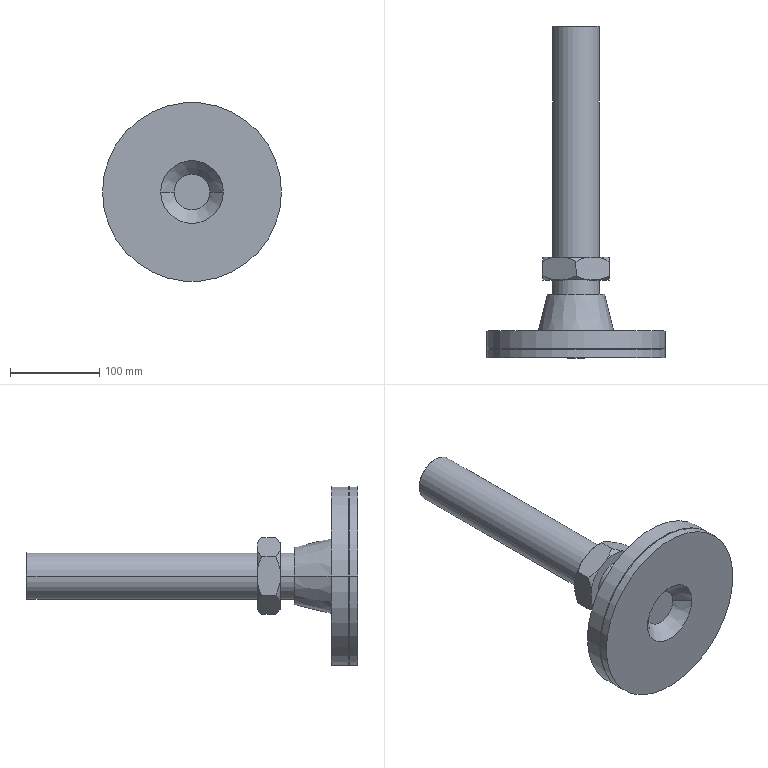Part | SolidWorks | features ICE 2, RevCut 2, Chamfer 1, Revolution 1 | 1 solid | 43 faces | box 200 x 371 x 200 mm | volume 1786955 mm3 | cone 22 | plane 13 | cylinder 8 | commonest cylinder face diameters 52 x4 200 x4
STEP:
#1=CARTESIAN_POINT('',(-25.,371.,0.));
#2=VERTEX_POINT('',#1);
#3=CARTESIAN_POINT('',(25.,371.,0.));
#4=VERTEX_POINT('',#3);
#5=CARTESIAN_POINT('',(0.,371.,0.));
#6=DIRECTION('',(0.,1.,0.));
#7=DIRECTION('',(1.,0.,0.));
#8=AXIS2_PLACEMENT_3D('',#5,#6,#7);
#9=CIRCLE('',#8,25.);
#10=EDGE_CURVE('',#2,#4,#9,.T.);
#11=ORIENTED_EDGE('',*,*,#10,.F.);
#12=CARTESIAN_POINT('',(-26.,370.,0.));
#13=VERTEX_POINT('',#12);
#14=CARTESIAN_POINT('',(-25.,371.,0.));
#15=DIRECTION('',(-0.7071,-0.7071,0.));
#16=VECTOR('',#15,1000.);
#17=LINE('',#14,#16);
#18=EDGE_CURVE('',#2,#13,#17,.T.);
#19=ORIENTED_EDGE('',*,*,#18,.T.);
#20=CARTESIAN_POINT('',(26.,370.,0.));
#21=VERTEX_POINT('',#20);
#22=CARTESIAN_POINT('',(0.,370.,0.));
#23=DIRECTION('',(0.,-1.,0.));
#24=DIRECTION('',(1.,0.,0.));
#25=AXIS2_PLACEMENT_3D('',#22,#23,#24);
#26=CIRCLE('',#25,26.);
#27=EDGE_CURVE('',#21,#13,#26,.T.);
#28=ORIENTED_EDGE('',*,*,#27,.F.);
#29=CARTESIAN_POINT('',(25.,371.,0.));
#30=DIRECTION('',(0.7071,-0.7071,0.));
#31=VECTOR('',#30,1000.);
#32=LINE('',#29,#31);
#33=EDGE_CURVE('',#4,#21,#32,.T.);
#34=ORIENTED_EDGE('',*,*,#33,.F.);
#35=EDGE_LOOP('',(#11,#19,#28,#34));
#36=FACE_OUTER_BOUND('',#35,.T.);
#37=CARTESIAN_POINT('',(0.,371.,0.));
#38=DIRECTION('',(0.,-1.,0.));
#39=DIRECTION('',(1.,0.,0.));
#40=AXIS2_PLACEMENT_3D('',#37,#38,#39);
#41=CONICAL_SURFACE('',#40,25.,0.7854);
#42=ADVANCED_FACE('',(#36),#41,.T.);
#43=CARTESIAN_POINT('',(-26.,112.6,0.));
#44=VERTEX_POINT('',#43);
#45=CARTESIAN_POINT('',(26.,112.6,0.));
#46=VERTEX_POINT('',#45);
#47=CARTESIAN_POINT('',(0.,112.6,0.));
#48=DIRECTION('',(0.,1.,0.));
#49=DIRECTION('',(-1.,0.,0.));
#50=AXIS2_PLACEMENT_3D('',#47,#48,#49);
#51=CIRCLE('',#50,26.);
#52=EDGE_CURVE('',#44,#46,#51,.T.);
#53=ORIENTED_EDGE('',*,*,#52,.T.);
#54=CARTESIAN_POINT('',(26.,371.,0.));
#55=DIRECTION('',(0.,1.,0.));
#56=VECTOR('',#55,1000.);
#57=LINE('',#54,#56);
#58=EDGE_CURVE('',#46,#21,#57,.T.);
#59=ORIENTED_EDGE('',*,*,#58,.T.);
#60=ORIENTED_EDGE('',*,*,#27,.T.);
#61=CARTESIAN_POINT('',(-26.,371.,0.));
#62=DIRECTION('',(0.,1.,0.));
#63=VECTOR('',#62,1000.);
#64=LINE('',#61,#63);
#65=EDGE_CURVE('',#44,#13,#64,.T.);
#66=ORIENTED_EDGE('',*,*,#65,.F.);
#67=EDGE_LOOP('',(#53,#59,#60,#66));
#68=FACE_OUTER_BOUND('',#67,.T.);
#69=CARTESIAN_POINT('',(0.,371.,0.));
#70=DIRECTION('',(0.,1.,0.));
#71=DIRECTION('',(-1.,0.,0.));
#72=AXIS2_PLACEMENT_3D('',#69,#70,#71);
#73=CYLINDRICAL_SURFACE('',#72,26.);
#74=ADVANCED_FACE('',(#68),#73,.T.);
#75=CARTESIAN_POINT('',(20.,15.,0.));
#76=VERTEX_POINT('',#75);
#77=CARTESIAN_POINT('',(-20.,15.,0.));
#78=VERTEX_POINT('',#77);
#79=CARTESIAN_POINT('',(0.,15.,0.));
#80=DIRECTION('',(0.,1.,0.));
#81=DIRECTION('',(-1.,0.,0.));
#82=AXIS2_PLACEMENT_3D('',#79,#80,#81);
#83=CIRCLE('',#82,20.);
#84=EDGE_CURVE('',#76,#78,#83,.T.);
#85=ORIENTED_EDGE('',*,*,#84,.T.);
#86=CARTESIAN_POINT('',(-35.,0.,0.));
#87=VERTEX_POINT('',#86);
#88=CARTESIAN_POINT('',(-20.,15.,0.));
#89=DIRECTION('',(-0.7071,-0.7071,0.));
#90=VECTOR('',#89,1000.);
#91=LINE('',#88,#90);
#92=EDGE_CURVE('',#78,#87,#91,.T.);
#93=ORIENTED_EDGE('',*,*,#92,.T.);
#94=CARTESIAN_POINT('',(35.,0.,0.));
#95=VERTEX_POINT('',#94);
#96=CARTESIAN_POINT('',(0.,0.,0.));
#97=DIRECTION('',(0.,1.,0.));
#98=DIRECTION('',(-1.,0.,0.));
#99=AXIS2_PLACEMENT_3D('',#96,#97,#98);
#100=CIRCLE('',#99,35.);
#101=EDGE_CURVE('',#95,#87,#100,.T.);
#102=ORIENTED_EDGE('',*,*,#101,.F.);
#103=CARTESIAN_POINT('',(20.,15.,0.));
#104=DIRECTION('',(0.7071,-0.7071,0.));
#105=VECTOR('',#104,1000.);
#106=LINE('',#103,#105);
#107=EDGE_CURVE('',#76,#95,#106,.T.);
#108=ORIENTED_EDGE('',*,*,#107,.F.);
#109=EDGE_LOOP('',(#85,#93,#102,#108));
#110=FACE_OUTER_BOUND('',#109,.T.);
#111=CARTESIAN_POINT('',(0.,15.,0.));
#112=DIRECTION('',(0.,-1.,0.));
#113=DIRECTION('',(1.,0.,0.));
#114=AXIS2_PLACEMENT_3D('',#111,#112,#113);
#115=CONICAL_SURFACE('',#114,20.,0.7854);
#116=ADVANCED_FACE('',(#110),#115,.F.);
#117=CARTESIAN_POINT('',(-32.,71.,0.));
#118=VERTEX_POINT('',#117);
#119=CARTESIAN_POINT('',(32.,71.,0.));
#120=VERTEX_POINT('',#119);
#121=CARTESIAN_POINT('',(0.,71.,0.));
#122=DIRECTION('',(0.,1.,0.));
#123=DIRECTION('',(-1.,0.,0.));
#124=AXIS2_PLACEMENT_3D('',#121,#122,#123);
#125=CIRCLE('',#124,32.);
#126=EDGE_CURVE('',#118,#120,#125,.T.);
#127=ORIENTED_EDGE('',*,*,#126,.F.);
#128=CARTESIAN_POINT('',(-42.,30.,0.));
#129=VERTEX_POINT('',#128);
#130=CARTESIAN_POINT('',(-42.,30.,0.));
#131=DIRECTION('',(-0.237,-0.9715,0.));
#132=VECTOR('',#131,1000.);
#133=LINE('',#130,#132);
#134=EDGE_CURVE('',#118,#129,#133,.T.);
#135=ORIENTED_EDGE('',*,*,#134,.T.);
#136=CARTESIAN_POINT('',(42.,30.,0.));
#137=VERTEX_POINT('',#136);
#138=CARTESIAN_POINT('',(0.,30.,0.));
#139=DIRECTION('',(0.,1.,0.));
#140=DIRECTION('',(-1.,0.,0.));
#141=AXIS2_PLACEMENT_3D('',#138,#139,#140);
#142=CIRCLE('',#141,42.);
#143=EDGE_CURVE('',#129,#137,#142,.T.);
#144=ORIENTED_EDGE('',*,*,#143,.T.);
#145=CARTESIAN_POINT('',(42.,30.,0.));
#146=DIRECTION('',(0.237,-0.9715,0.));
#147=VECTOR('',#146,1000.);
#148=LINE('',#145,#147);
#149=EDGE_CURVE('',#120,#137,#148,.T.);
#150=ORIENTED_EDGE('',*,*,#149,.F.);
#151=EDGE_LOOP('',(#127,#135,#144,#150));
#152=FACE_OUTER_BOUND('',#151,.T.);
#153=CARTESIAN_POINT('',(0.,30.,0.));
#154=DIRECTION('',(0.,-1.,0.));
#155=DIRECTION('',(1.,0.,0.));
#156=AXIS2_PLACEMENT_3D('',#153,#154,#155);
#157=CONICAL_SURFACE('',#156,42.,0.2392);
#158=ADVANCED_FACE('',(#152),#157,.T.);
#159=CARTESIAN_POINT('',(-100.,10.5,0.));
#160=VERTEX_POINT('',#159);
#161=CARTESIAN_POINT('',(100.,10.5,0.));
#162=VERTEX_POINT('',#161);
#163=CARTESIAN_POINT('',(0.,10.5,0.));
#164=DIRECTION('',(0.,1.,0.));
#165=DIRECTION('',(-1.,0.,0.));
#166=AXIS2_PLACEMENT_3D('',#163,#164,#165);
#167=CIRCLE('',#166,100.);
#168=EDGE_CURVE('',#160,#162,#167,.T.);
#169=ORIENTED_EDGE('',*,*,#168,.T.);
#170=CARTESIAN_POINT('',(100.,30.,0.));
#171=VERTEX_POINT('',#170);
#172=CARTESIAN_POINT('',(100.,371.,0.));
#173=DIRECTION('',(0.,1.,0.));
#174=VECTOR('',#173,1000.);
#175=LINE('',#172,#174);
#176=EDGE_CURVE('',#162,#171,#175,.T.);
#177=ORIENTED_EDGE('',*,*,#176,.T.);
#178=CARTESIAN_POINT('',(-100.,30.,0.));
#179=VERTEX_POINT('',#178);
#180=CARTESIAN_POINT('',(0.,30.,0.));
#181=DIRECTION('',(0.,1.,0.));
#182=DIRECTION('',(-1.,0.,0.));
#183=AXIS2_PLACEMENT_3D('',#180,#181,#182);
#184=CIRCLE('',#183,100.);
#185=EDGE_CURVE('',#179,#171,#184,.T.);
#186=ORIENTED_EDGE('',*,*,#185,.F.);
#187=CARTESIAN_POINT('',(-100.,371.,0.));
#188=DIRECTION('',(0.,1.,0.));
#189=VECTOR('',#188,1000.);
#190=LINE('',#187,#189);
#191=EDGE_CURVE('',#160,#179,#190,.T.);
#192=ORIENTED_EDGE('',*,*,#191,.F.);
#193=EDGE_LOOP('',(#169,#177,#186,#192));
#194=FACE_OUTER_BOUND('',#193,.T.);
#195=CARTESIAN_POINT('',(0.,371.,0.));
#196=DIRECTION('',(0.,1.,0.));
#197=DIRECTION('',(-1.,0.,0.));
#198=AXIS2_PLACEMENT_3D('',#195,#196,#197);
#199=CYLINDRICAL_SURFACE('',#198,100.);
#200=ADVANCED_FACE('',(#194),#199,.T.);
#201=CARTESIAN_POINT('',(-99.5,10.,0.));
#202=VERTEX_POINT('',#201);
#203=CARTESIAN_POINT('',(99.5,10.,0.));
#204=VERTEX_POINT('',#203);
#205=CARTESIAN_POINT('',(0.,10.,0.));
#206=DIRECTION('',(0.,1.,0.));
#207=DIRECTION('',(-1.,0.,0.));
#208=AXIS2_PLACEMENT_3D('',#205,#206,#207);
#209=CIRCLE('',#208,99.5);
#210=EDGE_CURVE('',#202,#204,#209,.T.);
#211=ORIENTED_EDGE('',*,*,#210,.T.);
#212=CARTESIAN_POINT('',(99.5,10.,0.));
#213=DIRECTION('',(0.7071,0.7071,0.));
#214=VECTOR('',#213,1000.);
#215=LINE('',#212,#214);
#216=EDGE_CURVE('',#204,#162,#215,.T.);
#217=ORIENTED_EDGE('',*,*,#216,.T.);
#218=ORIENTED_EDGE('',*,*,#168,.F.);
#219=CARTESIAN_POINT('',(-99.5,10.,0.));
#220=DIRECTION('',(-0.7071,0.7071,0.));
#221=VECTOR('',#220,1000.);
#222=LINE('',#219,#221);
#223=EDGE_CURVE('',#202,#160,#222,.T.);
#224=ORIENTED_EDGE('',*,*,#223,.F.);
#225=EDGE_LOOP('',(#211,#217,#218,#224));
#226=FACE_OUTER_BOUND('',#225,.T.);
#227=CARTESIAN_POINT('',(0.,10.,0.));
#228=DIRECTION('',(0.,1.,0.));
#229=DIRECTION('',(-1.,0.,0.));
#230=AXIS2_PLACEMENT_3D('',#227,#228,#229);
#231=CONICAL_SURFACE('',#230,99.5,0.7854);
#232=ADVANCED_FACE('',(#226),#231,.T.);
#233=ORIENTED_EDGE('',*,*,#210,.F.);
#234=CARTESIAN_POINT('',(-100.,9.5,0.));
#235=VERTEX_POINT('',#234);
#236=CARTESIAN_POINT('',(-100.,9.5,0.));
#237=DIRECTION('',(-0.7071,-0.7071,0.));
#238=VECTOR('',#237,1000.);
#239=LINE('',#236,#238);
#240=EDGE_CURVE('',#202,#235,#239,.T.);
#241=ORIENTED_EDGE('',*,*,#240,.T.);
#242=CARTESIAN_POINT('',(100.,9.5,0.));
#243=VERTEX_POINT('',#242);
#244=CARTESIAN_POINT('',(0.,9.5,0.));
#245=DIRECTION('',(0.,1.,0.));
#246=DIRECTION('',(-1.,0.,0.));
#247=AXIS2_PLACEMENT_3D('',#244,#245,#246);
#248=CIRCLE('',#247,100.);
#249=EDGE_CURVE('',#235,#243,#248,.T.);
#250=ORIENTED_EDGE('',*,*,#249,.T.);
#251=CARTESIAN_POINT('',(100.,9.5,0.));
#252=DIRECTION('',(0.7071,-0.7071,0.));
#253=VECTOR('',#252,1000.);
#254=LINE('',#251,#253);
#255=EDGE_CURVE('',#204,#243,#254,.T.);
#256=ORIENTED_EDGE('',*,*,#255,.F.);
#257=EDGE_LOOP('',(#233,#241,#250,#256));
#258=FACE_OUTER_BOUND('',#257,.T.);
#259=CARTESIAN_POINT('',(0.,9.5,0.));
#260=DIRECTION('',(0.,-1.,0.));
#261=DIRECTION('',(1.,0.,0.));
#262=AXIS2_PLACEMENT_3D('',#259,#260,#261);
#263=CONICAL_SURFACE('',#262,100.,0.7854);
#264=ADVANCED_FACE('',(#258),#263,.T.);
#265=CARTESIAN_POINT('',(-100.,0.,0.));
#266=VERTEX_POINT('',#265);
#267=CARTESIAN_POINT('',(100.,0.,0.));
#268=VERTEX_POINT('',#267);
#269=CARTESIAN_POINT('',(0.,0.,0.));
#270=DIRECTION('',(0.,1.,0.));
#271=DIRECTION('',(-1.,0.,0.));
#272=AXIS2_PLACEMENT_3D('',#269,#270,#271);
#273=CIRCLE('',#272,100.);
#274=EDGE_CURVE('',#266,#268,#273,.T.);
#275=ORIENTED_EDGE('',*,*,#274,.T.);
#276=CARTESIAN_POINT('',(100.,371.,0.));
#277=DIRECTION('',(0.,1.,0.));
#278=VECTOR('',#277,1000.);
#279=LINE('',#276,#278);
#280=EDGE_CURVE('',#268,#243,#279,.T.);
#281=ORIENTED_EDGE('',*,*,#280,.T.);
#282=ORIENTED_EDGE('',*,*,#249,.F.);
#283=CARTESIAN_POINT('',(-100.,371.,0.));
#284=DIRECTION('',(0.,1.,0.));
#285=VECTOR('',#284,1000.);
#286=LINE('',#283,#285);
#287=EDGE_CURVE('',#266,#235,#286,.T.);
#288=ORIENTED_EDGE('',*,*,#287,.F.);
#289=EDGE_LOOP('',(#275,#281,#282,#288));
#290=FACE_OUTER_BOUND('',#289,.T.);
#291=CARTESIAN_POINT('',(0.,371.,0.));
#292=DIRECTION('',(0.,1.,0.));
#293=DIRECTION('',(-1.,0.,0.));
#294=AXIS2_PLACEMENT_3D('',#291,#292,#293);
#295=CYLINDRICAL_SURFACE('',#294,100.);
#296=ADVANCED_FACE('',(#290),#295,.T.);
#297=CARTESIAN_POINT('',(-26.,71.,0.));
#298=VERTEX_POINT('',#297);
#299=CARTESIAN_POINT('',(26.,71.,0.));
#300=VERTEX_POINT('',#299);
#301=CARTESIAN_POINT('',(0.,71.,0.));
#302=DIRECTION('',(0.,1.,0.));
#303=DIRECTION('',(-1.,0.,0.));
#304=AXIS2_PLACEMENT_3D('',#301,#302,#303);
#305=CIRCLE('',#304,26.);
#306=EDGE_CURVE('',#298,#300,#305,.T.);
#307=ORIENTED_EDGE('',*,*,#306,.T.);
#308=CARTESIAN_POINT('',(26.,87.,0.));
#309=VERTEX_POINT('',#308);
#310=CARTESIAN_POINT('',(26.,371.,0.));
#311=DIRECTION('',(0.,1.,0.));
#312=VECTOR('',#311,1000.);
#313=LINE('',#310,#312);
#314=EDGE_CURVE('',#300,#309,#313,.T.);
#315=ORIENTED_EDGE('',*,*,#314,.T.);
#316=CARTESIAN_POINT('',(-26.,87.,0.));
#317=VERTEX_POINT('',#316);
#318=CARTESIAN_POINT('',(0.,87.,0.));
#319=DIRECTION('',(0.,1.,0.));
#320=DIRECTION('',(0.,0.,1.));
#321=AXIS2_PLACEMENT_3D('',#318,#319,#320);
#322=CIRCLE('',#321,26.);
#323=EDGE_CURVE('',#317,#309,#322,.T.);
#324=ORIENTED_EDGE('',*,*,#323,.F.);
#325=CARTESIAN_POINT('',(-26.,371.,0.));
#326=DIRECTION('',(0.,1.,0.));
#327=VECTOR('',#326,1000.);
#328=LINE('',#325,#327);
#329=EDGE_CURVE('',#298,#317,#328,.T.);
#330=ORIENTED_EDGE('',*,*,#329,.F.);
#331=EDGE_LOOP('',(#307,#315,#324,#330));
#332=FACE_OUTER_BOUND('',#331,.T.);
#333=CARTESIAN_POINT('',(0.,371.,0.));
#334=DIRECTION('',(0.,1.,0.));
#335=DIRECTION('',(-1.,0.,0.));
#336=AXIS2_PLACEMENT_3D('',#333,#334,#335);
#337=CYLINDRICAL_SURFACE('',#336,26.);
#338=ADVANCED_FACE('',(#332),#337,.T.);
#339=ORIENTED_EDGE('',*,*,#52,.F.);
#340=CARTESIAN_POINT('',(0.,112.6,0.));
#341=DIRECTION('',(0.,1.,0.));
#342=DIRECTION('',(-1.,0.,0.));
#343=AXIS2_PLACEMENT_3D('',#340,#341,#342);
#344=CIRCLE('',#343,26.);
#345=EDGE_CURVE('',#46,#44,#344,.T.);
#346=ORIENTED_EDGE('',*,*,#345,.F.);
#347=EDGE_LOOP('',(#339,#346));
#348=FACE_BOUND('',#347,.T.);
#349=CARTESIAN_POINT('',(-24.996,112.6,28.408));
#350=VERTEX_POINT('',#349);
#351=CARTESIAN_POINT('',(-37.1,112.6,7.444));
#352=VERTEX_POINT('',#351);
#353=CARTESIAN_POINT('',(0.,112.6,0.));
#354=DIRECTION('',(0.,-1.,0.));
#355=DIRECTION('',(1.,0.,0.));
#356=AXIS2_PLACEMENT_3D('',#353,#354,#355);
#357=CIRCLE('',#356,37.839);
#358=EDGE_CURVE('',#350,#352,#357,.T.);
#359=ORIENTED_EDGE('',*,*,#358,.F.);
#360=CARTESIAN_POINT('',(-12.104,112.6,35.851));
#361=VERTEX_POINT('',#360);
#362=CARTESIAN_POINT('',(-37.1,112.6,21.42));
#363=DIRECTION('',(0.866,0.,0.5));
#364=VECTOR('',#363,1000.);
#365=LINE('',#362,#364);
#366=EDGE_CURVE('',#350,#361,#365,.T.);
#367=ORIENTED_EDGE('',*,*,#366,.T.);
#368=CARTESIAN_POINT('',(12.104,112.6,35.851));
#369=VERTEX_POINT('',#368);
#370=CARTESIAN_POINT('',(0.,112.6,0.));
#371=DIRECTION('',(0.,-1.,0.));
#372=DIRECTION('',(1.,0.,0.));
#373=AXIS2_PLACEMENT_3D('',#370,#371,#372);
#374=CIRCLE('',#373,37.839);
#375=EDGE_CURVE('',#369,#361,#374,.T.);
#376=ORIENTED_EDGE('',*,*,#375,.F.);
#377=CARTESIAN_POINT('',(24.996,112.6,28.408));
#378=VERTEX_POINT('',#377);
#379=CARTESIAN_POINT('',(0.,112.6,42.839));
#380=DIRECTION('',(0.866,0.,-0.5));
#381=VECTOR('',#380,1000.);
#382=LINE('',#379,#381);
#383=EDGE_CURVE('',#369,#378,#382,.T.);
#384=ORIENTED_EDGE('',*,*,#383,.T.);
#385=CARTESIAN_POINT('',(37.1,112.6,7.444));
#386=VERTEX_POINT('',#385);
#387=CARTESIAN_POINT('',(0.,112.6,0.));
#388=DIRECTION('',(0.,-1.,0.));
#389=DIRECTION('',(1.,0.,0.));
#390=AXIS2_PLACEMENT_3D('',#387,#388,#389);
#391=CIRCLE('',#390,37.839);
#392=EDGE_CURVE('',#386,#378,#391,.T.);
#393=ORIENTED_EDGE('',*,*,#392,.F.);
#394=CARTESIAN_POINT('',(37.1,112.6,-7.444));
#395=VERTEX_POINT('',#394);
#396=CARTESIAN_POINT('',(37.1,112.6,21.42));
#397=DIRECTION('',(0.,0.,-1.));
#398=VECTOR('',#397,1000.);
#399=LINE('',#396,#398);
#400=EDGE_CURVE('',#386,#395,#399,.T.);
#401=ORIENTED_EDGE('',*,*,#400,.T.);
#402=CARTESIAN_POINT('',(24.996,112.6,-28.408));
#403=VERTEX_POINT('',#402);
#404=CARTESIAN_POINT('',(0.,112.6,0.));
#405=DIRECTION('',(0.,-1.,0.));
#406=DIRECTION('',(1.,0.,0.));
#407=AXIS2_PLACEMENT_3D('',#404,#405,#406);
#408=CIRCLE('',#407,37.839);
#409=EDGE_CURVE('',#403,#395,#408,.T.);
#410=ORIENTED_EDGE('',*,*,#409,.F.);
#411=CARTESIAN_POINT('',(12.104,112.6,-35.851));
#412=VERTEX_POINT('',#411);
#413=CARTESIAN_POINT('',(37.1,112.6,-21.42));
#414=DIRECTION('',(-0.866,0.,-0.5));
#415=VECTOR('',#414,1000.);
#416=LINE('',#413,#415);
#417=EDGE_CURVE('',#403,#412,#416,.T.);
#418=ORIENTED_EDGE('',*,*,#417,.T.);
#419=CARTESIAN_POINT('',(-12.104,112.6,-35.851));
#420=VERTEX_POINT('',#419);
#421=CARTESIAN_POINT('',(0.,112.6,0.));
#422=DIRECTION('',(0.,-1.,0.));
#423=DIRECTION('',(1.,0.,0.));
#424=AXIS2_PLACEMENT_3D('',#421,#422,#423);
#425=CIRCLE('',#424,37.839);
#426=EDGE_CURVE('',#420,#412,#425,.T.);
#427=ORIENTED_EDGE('',*,*,#426,.F.);
#428=CARTESIAN_POINT('',(-24.996,112.6,-28.408));
#429=VERTEX_POINT('',#428);
#430=CARTESIAN_POINT('',(0.,112.6,-42.839));
#431=DIRECTION('',(-0.866,0.,0.5));
#432=VECTOR('',#431,1000.);
#433=LINE('',#430,#432);
#434=EDGE_CURVE('',#420,#429,#433,.T.);
#435=ORIENTED_EDGE('',*,*,#434,.T.);
#436=CARTESIAN_POINT('',(-37.1,112.6,-7.444));
#437=VERTEX_POINT('',#436);
#438=CARTESIAN_POINT('',(0.,112.6,0.));
#439=DIRECTION('',(0.,-1.,0.));
#440=DIRECTION('',(1.,0.,0.));
#441=AXIS2_PLACEMENT_3D('',#438,#439,#440);
#442=CIRCLE('',#441,37.839);
#443=EDGE_CURVE('',#437,#429,#442,.T.);
#444=ORIENTED_EDGE('',*,*,#443,.F.);
#445=CARTESIAN_POINT('',(-37.1,112.6,-21.42));
#446=DIRECTION('',(0.,0.,1.));
#447=VECTOR('',#446,1000.);
#448=LINE('',#445,#447);
#449=EDGE_CURVE('',#437,#352,#448,.T.);
#450=ORIENTED_EDGE('',*,*,#449,.T.);
#451=EDGE_LOOP('',(#359,#367,#376,#384,#393,#401,#410,#418,#427,#435,#444,#450));
#452=FACE_OUTER_BOUND('',#451,.T.);
#453=CARTESIAN_POINT('',(0.,112.6,0.));
#454=DIRECTION('',(0.,1.,0.));
#455=DIRECTION('',(0.,0.,1.));
#456=AXIS2_PLACEMENT_3D('',#453,#454,#455);
#457=PLANE('',#456);
#458=ADVANCED_FACE('',(#348,#452),#457,.T.);
#459=ORIENTED_EDGE('',*,*,#314,.F.);
#460=CARTESIAN_POINT('',(0.,71.,0.));
#461=DIRECTION('',(0.,1.,0.));
#462=DIRECTION('',(-1.,0.,0.));
#463=AXIS2_PLACEMENT_3D('',#460,#461,#462);
#464=CIRCLE('',#463,26.);
#465=EDGE_CURVE('',#300,#298,#464,.T.);
#466=ORIENTED_EDGE('',*,*,#465,.T.);
#467=ORIENTED_EDGE('',*,*,#329,.T.);
#468=CARTESIAN_POINT('',(0.,87.,0.));
#469=DIRECTION('',(0.,1.,0.));
#470=DIRECTION('',(0.,0.,1.));
#471=AXIS2_PLACEMENT_3D('',#468,#469,#470);
#472=CIRCLE('',#471,26.);
#473=EDGE_CURVE('',#309,#317,#472,.T.);
#474=ORIENTED_EDGE('',*,*,#473,.F.);
#475=EDGE_LOOP('',(#459,#466,#467,#474));
#476=FACE_OUTER_BOUND('',#475,.T.);
#477=CARTESIAN_POINT('',(0.,371.,0.));
#478=DIRECTION('',(0.,1.,0.));
#479=DIRECTION('',(-1.,0.,0.));
#480=AXIS2_PLACEMENT_3D('',#477,#478,#479);
#481=CYLINDRICAL_SURFACE('',#480,26.);
#482=ADVANCED_FACE('',(#476),#481,.T.);
#483=ORIENTED_EDGE('',*,*,#280,.F.);
#484=CARTESIAN_POINT('',(0.,0.,0.));
#485=DIRECTION('',(0.,1.,0.));
#486=DIRECTION('',(-1.,0.,0.));
#487=AXIS2_PLACEMENT_3D('',#484,#485,#486);
#488=CIRCLE('',#487,100.);
#489=EDGE_CURVE('',#268,#266,#488,.T.);
#490=ORIENTED_EDGE('',*,*,#489,.T.);
#491=ORIENTED_EDGE('',*,*,#287,.T.);
#492=CARTESIAN_POINT('',(0.,9.5,0.));
#493=DIRECTION('',(0.,1.,0.));
#494=DIRECTION('',(-1.,0.,0.));
#495=AXIS2_PLACEMENT_3D('',#492,#493,#494);
#496=CIRCLE('',#495,100.);
#497=EDGE_CURVE('',#243,#235,#496,.T.);
#498=ORIENTED_EDGE('',*,*,#497,.F.);
#499=EDGE_LOOP('',(#483,#490,#491,#498));
#500=FACE_OUTER_BOUND('',#499,.T.);
#501=CARTESIAN_POINT('',(0.,371.,0.));
#502=DIRECTION('',(0.,1.,0.));
#503=DIRECTION('',(-1.,0.,0.));
#504=AXIS2_PLACEMENT_3D('',#501,#502,#503);
#505=CYLINDRICAL_SURFACE('',#504,100.);
#506=ADVANCED_FACE('',(#500),#505,.T.);
#507=ORIENTED_EDGE('',*,*,#240,.F.);
#508=CARTESIAN_POINT('',(0.,10.,0.));
#509=DIRECTION('',(0.,1.,0.));
#510=DIRECTION('',(-1.,0.,0.));
#511=AXIS2_PLACEMENT_3D('',#508,#509,#510);
#512=CIRCLE('',#511,99.5);
#513=EDGE_CURVE('',#204,#202,#512,.T.);
#514=ORIENTED_EDGE('',*,*,#513,.F.);
#515=ORIENTED_EDGE('',*,*,#255,.T.);
#516=ORIENTED_EDGE('',*,*,#497,.T.);
#517=EDGE_LOOP('',(#507,#514,#515,#516));
#518=FACE_OUTER_BOUND('',#517,.T.);
#519=CARTESIAN_POINT('',(0.,9.5,0.));
#520=DIRECTION('',(0.,-1.,0.));
#521=DIRECTION('',(1.,0.,0.));
#522=AXIS2_PLACEMENT_3D('',#519,#520,#521);
#523=CONICAL_SURFACE('',#522,100.,0.7854);
#524=ADVANCED_FACE('',(#518),#523,.T.);
#525=ORIENTED_EDGE('',*,*,#216,.F.);
#526=ORIENTED_EDGE('',*,*,#513,.T.);
#527=ORIENTED_EDGE('',*,*,#223,.T.);
#528=CARTESIAN_POINT('',(0.,10.5,0.));
#529=DIRECTION('',(0.,1.,0.));
#530=DIRECTION('',(-1.,0.,0.));
#531=AXIS2_PLACEMENT_3D('',#528,#529,#530);
#532=CIRCLE('',#531,100.);
#533=EDGE_CURVE('',#162,#160,#532,.T.);
#534=ORIENTED_EDGE('',*,*,#533,.F.);
#535=EDGE_LOOP('',(#525,#526,#527,#534));
#536=FACE_OUTER_BOUND('',#535,.T.);
#537=CARTESIAN_POINT('',(0.,10.,0.));
#538=DIRECTION('',(0.,1.,0.));
#539=DIRECTION('',(-1.,0.,0.));
#540=AXIS2_PLACEMENT_3D('',#537,#538,#539);
#541=CONICAL_SURFACE('',#540,99.5,0.7854);
#542=ADVANCED_FACE('',(#536),#541,.T.);
#543=ORIENTED_EDGE('',*,*,#176,.F.);
#544=ORIENTED_EDGE('',*,*,#533,.T.);
#545=ORIENTED_EDGE('',*,*,#191,.T.);
#546=CARTESIAN_POINT('',(0.,30.,0.));
#547=DIRECTION('',(0.,1.,0.));
#548=DIRECTION('',(-1.,0.,0.));
#549=AXIS2_PLACEMENT_3D('',#546,#547,#548);
#550=CIRCLE('',#549,100.);
#551=EDGE_CURVE('',#171,#179,#550,.T.);
#552=ORIENTED_EDGE('',*,*,#551,.F.);
#553=EDGE_LOOP('',(#543,#544,#545,#552));
#554=FACE_OUTER_BOUND('',#553,.T.);
#555=CARTESIAN_POINT('',(0.,371.,0.));
#556=DIRECTION('',(0.,1.,0.));
#557=DIRECTION('',(-1.,0.,0.));
#558=AXIS2_PLACEMENT_3D('',#555,#556,#557);
#559=CYLINDRICAL_SURFACE('',#558,100.);
#560=ADVANCED_FACE('',(#554),#559,.T.);
#561=CARTESIAN_POINT('',(0.,30.,0.));
#562=DIRECTION('',(0.,1.,0.));
#563=DIRECTION('',(-1.,0.,0.));
#564=AXIS2_PLACEMENT_3D('',#561,#562,#563);
#565=CIRCLE('',#564,42.);
#566=EDGE_CURVE('',#137,#129,#565,.T.);
#567=ORIENTED_EDGE('',*,*,#566,.F.);
#568=ORIENTED_EDGE('',*,*,#143,.F.);
#569=EDGE_LOOP('',(#567,#568));
#570=FACE_BOUND('',#569,.T.);
#571=ORIENTED_EDGE('',*,*,#185,.T.);
#572=ORIENTED_EDGE('',*,*,#551,.T.);
#573=EDGE_LOOP('',(#571,#572));
#574=FACE_OUTER_BOUND('',#573,.T.);
#575=CARTESIAN_POINT('',(100.,30.,0.));
#576=DIRECTION('',(0.,-1.,0.));
#577=DIRECTION('',(1.,0.,0.));
#578=AXIS2_PLACEMENT_3D('',#575,#576,#577);
#579=PLANE('',#578);
#580=ADVANCED_FACE('',(#570,#574),#579,.F.);
#581=ORIENTED_EDGE('',*,*,#134,.F.);
#582=CARTESIAN_POINT('',(0.,71.,0.));
#583=DIRECTION('',(0.,1.,0.));
#584=DIRECTION('',(-1.,0.,0.));
#585=AXIS2_PLACEMENT_3D('',#582,#583,#584);
#586=CIRCLE('',#585,32.);
#587=EDGE_CURVE('',#120,#118,#586,.T.);
#588=ORIENTED_EDGE('',*,*,#587,.F.);
#589=ORIENTED_EDGE('',*,*,#149,.T.);
#590=ORIENTED_EDGE('',*,*,#566,.T.);
#591=EDGE_LOOP('',(#581,#588,#589,#590));
#592=FACE_OUTER_BOUND('',#591,.T.);
#593=CARTESIAN_POINT('',(0.,30.,0.));
#594=DIRECTION('',(0.,-1.,0.));
#595=DIRECTION('',(1.,0.,0.));
#596=AXIS2_PLACEMENT_3D('',#593,#594,#595);
#597=CONICAL_SURFACE('',#596,42.,0.2392);
#598=ADVANCED_FACE('',(#592),#597,.T.);
#599=ORIENTED_EDGE('',*,*,#306,.F.);
#600=ORIENTED_EDGE('',*,*,#465,.F.);
#601=EDGE_LOOP('',(#599,#600));
#602=FACE_BOUND('',#601,.T.);
#603=ORIENTED_EDGE('',*,*,#587,.T.);
#604=ORIENTED_EDGE('',*,*,#126,.T.);
#605=EDGE_LOOP('',(#603,#604));
#606=FACE_OUTER_BOUND('',#605,.T.);
#607=CARTESIAN_POINT('',(32.,71.,0.));
#608=DIRECTION('',(0.,-1.,0.));
#609=DIRECTION('',(1.,0.,0.));
#610=AXIS2_PLACEMENT_3D('',#607,#608,#609);
#611=PLANE('',#610);
#612=ADVANCED_FACE('',(#602,#606),#611,.F.);
#613=ORIENTED_EDGE('',*,*,#84,.F.);
#614=CARTESIAN_POINT('',(0.,15.,0.));
#615=DIRECTION('',(0.,1.,0.));
#616=DIRECTION('',(-1.,0.,0.));
#617=AXIS2_PLACEMENT_3D('',#614,#615,#616);
#618=CIRCLE('',#617,20.);
#619=EDGE_CURVE('',#78,#76,#618,.T.);
#620=ORIENTED_EDGE('',*,*,#619,.F.);
#621=EDGE_LOOP('',(#613,#620));
#622=FACE_OUTER_BOUND('',#621,.T.);
#623=CARTESIAN_POINT('',(0.,15.,0.));
#624=DIRECTION('',(0.,1.,0.));
#625=DIRECTION('',(-1.,0.,0.));
#626=AXIS2_PLACEMENT_3D('',#623,#624,#625);
#627=PLANE('',#626);
#628=ADVANCED_FACE('',(#622),#627,.F.);
#629=ORIENTED_EDGE('',*,*,#92,.F.);
#630=ORIENTED_EDGE('',*,*,#619,.T.);
#631=ORIENTED_EDGE('',*,*,#107,.T.);
#632=CARTESIAN_POINT('',(0.,0.,0.));
#633=DIRECTION('',(0.,1.,0.));
#634=DIRECTION('',(-1.,0.,0.));
#635=AXIS2_PLACEMENT_3D('',#632,#633,#634);
#636=CIRCLE('',#635,35.);
#637=EDGE_CURVE('',#87,#95,#636,.T.);
#638=ORIENTED_EDGE('',*,*,#637,.F.);
#639=EDGE_LOOP('',(#629,#630,#631,#638));
#640=FACE_OUTER_BOUND('',#639,.T.);
#641=CARTESIAN_POINT('',(0.,15.,0.));
#642=DIRECTION('',(0.,-1.,0.));
#643=DIRECTION('',(1.,0.,0.));
#644=AXIS2_PLACEMENT_3D('',#641,#642,#643);
#645=CONICAL_SURFACE('',#644,20.,0.7854);
#646=ADVANCED_FACE('',(#640),#645,.F.);
#647=ORIENTED_EDGE('',*,*,#274,.F.);
#648=ORIENTED_EDGE('',*,*,#489,.F.);
#649=EDGE_LOOP('',(#647,#648));
#650=FACE_OUTER_BOUND('',#649,.T.);
#651=ORIENTED_EDGE('',*,*,#101,.T.);
#652=ORIENTED_EDGE('',*,*,#637,.T.);
#653=EDGE_LOOP('',(#651,#652));
#654=FACE_BOUND('',#653,.T.);
#655=CARTESIAN_POINT('',(35.,0.,0.));
#656=DIRECTION('',(0.,1.,0.));
#657=DIRECTION('',(-1.,0.,0.));
#658=AXIS2_PLACEMENT_3D('',#655,#656,#657);
#659=PLANE('',#658);
#660=ADVANCED_FACE('',(#650,#654),#659,.F.);
#661=CARTESIAN_POINT('',(-24.996,87.,28.408));
#662=VERTEX_POINT('',#661);
#663=CARTESIAN_POINT('',(-12.104,87.,35.851));
#664=VERTEX_POINT('',#663);
#665=CARTESIAN_POINT('',(-37.1,87.,21.42));
#666=DIRECTION('',(0.866,0.,0.5));
#667=VECTOR('',#666,1000.);
#668=LINE('',#665,#667);
#669=EDGE_CURVE('',#662,#664,#668,.T.);
#670=ORIENTED_EDGE('',*,*,#669,.F.);
#671=CARTESIAN_POINT('',(-37.1,87.,7.444));
#672=VERTEX_POINT('',#671);
#673=CARTESIAN_POINT('',(0.,87.,0.));
#674=DIRECTION('',(0.,-1.,0.));
#675=DIRECTION('',(1.,0.,0.));
#676=AXIS2_PLACEMENT_3D('',#673,#674,#675);
#677=CIRCLE('',#676,37.839);
#678=EDGE_CURVE('',#662,#672,#677,.T.);
#679=ORIENTED_EDGE('',*,*,#678,.T.);
#680=CARTESIAN_POINT('',(-37.1,87.,-7.444));
#681=VERTEX_POINT('',#680);
#682=CARTESIAN_POINT('',(-37.1,87.,-21.42));
#683=DIRECTION('',(0.,0.,1.));
#684=VECTOR('',#683,1000.);
#685=LINE('',#682,#684);
#686=EDGE_CURVE('',#681,#672,#685,.T.);
#687=ORIENTED_EDGE('',*,*,#686,.F.);
#688=CARTESIAN_POINT('',(-24.996,87.,-28.408));
#689=VERTEX_POINT('',#688);
#690=CARTESIAN_POINT('',(0.,87.,0.));
#691=DIRECTION('',(0.,-1.,0.));
#692=DIRECTION('',(1.,0.,0.));
#693=AXIS2_PLACEMENT_3D('',#690,#691,#692);
#694=CIRCLE('',#693,37.839);
#695=EDGE_CURVE('',#681,#689,#694,.T.);
#696=ORIENTED_EDGE('',*,*,#695,.T.);
#697=CARTESIAN_POINT('',(-12.104,87.,-35.851));
#698=VERTEX_POINT('',#697);
#699=CARTESIAN_POINT('',(0.,87.,-42.839));
#700=DIRECTION('',(-0.866,0.,0.5));
#701=VECTOR('',#700,1000.);
#702=LINE('',#699,#701);
#703=EDGE_CURVE('',#698,#689,#702,.T.);
#704=ORIENTED_EDGE('',*,*,#703,.F.);
#705=CARTESIAN_POINT('',(12.104,87.,-35.851));
#706=VERTEX_POINT('',#705);
#707=CARTESIAN_POINT('',(0.,87.,0.));
#708=DIRECTION('',(0.,-1.,0.));
#709=DIRECTION('',(1.,0.,0.));
#710=AXIS2_PLACEMENT_3D('',#707,#708,#709);
#711=CIRCLE('',#710,37.839);
#712=EDGE_CURVE('',#698,#706,#711,.T.);
#713=ORIENTED_EDGE('',*,*,#712,.T.);
#714=CARTESIAN_POINT('',(24.996,87.,-28.408));
#715=VERTEX_POINT('',#714);
#716=CARTESIAN_POINT('',(37.1,87.,-21.42));
#717=DIRECTION('',(-0.866,0.,-0.5));
#718=VECTOR('',#717,1000.);
#719=LINE('',#716,#718);
#720=EDGE_CURVE('',#715,#706,#719,.T.);
#721=ORIENTED_EDGE('',*,*,#720,.F.);
#722=CARTESIAN_POINT('',(37.1,87.,-7.444));
#723=VERTEX_POINT('',#722);
#724=CARTESIAN_POINT('',(0.,87.,0.));
#725=DIRECTION('',(0.,-1.,0.));
#726=DIRECTION('',(1.,0.,0.));
#727=AXIS2_PLACEMENT_3D('',#724,#725,#726);
#728=CIRCLE('',#727,37.839);
#729=EDGE_CURVE('',#715,#723,#728,.T.);
#730=ORIENTED_EDGE('',*,*,#729,.T.);
#731=CARTESIAN_POINT('',(37.1,87.,7.444));
#732=VERTEX_POINT('',#731);
#733=CARTESIAN_POINT('',(37.1,87.,21.42));
#734=DIRECTION('',(0.,0.,-1.));
#735=VECTOR('',#734,1000.);
#736=LINE('',#733,#735);
#737=EDGE_CURVE('',#732,#723,#736,.T.);
#738=ORIENTED_EDGE('',*,*,#737,.F.);
#739=CARTESIAN_POINT('',(24.996,87.,28.408));
#740=VERTEX_POINT('',#739);
#741=CARTESIAN_POINT('',(0.,87.,0.));
#742=DIRECTION('',(0.,-1.,0.));
#743=DIRECTION('',(1.,0.,0.));
#744=AXIS2_PLACEMENT_3D('',#741,#742,#743);
#745=CIRCLE('',#744,37.839);
#746=EDGE_CURVE('',#732,#740,#745,.T.);
#747=ORIENTED_EDGE('',*,*,#746,.T.);
#748=CARTESIAN_POINT('',(12.104,87.,35.851));
#749=VERTEX_POINT('',#748);
#750=CARTESIAN_POINT('',(0.,87.,42.839));
#751=DIRECTION('',(0.866,0.,-0.5));
#752=VECTOR('',#751,1000.);
#753=LINE('',#750,#752);
#754=EDGE_CURVE('',#749,#740,#753,.T.);
#755=ORIENTED_EDGE('',*,*,#754,.F.);
#756=CARTESIAN_POINT('',(0.,87.,0.));
#757=DIRECTION('',(0.,-1.,0.));
#758=DIRECTION('',(1.,0.,0.));
#759=AXIS2_PLACEMENT_3D('',#756,#757,#758);
#760=CIRCLE('',#759,37.839);
#761=EDGE_CURVE('',#749,#664,#760,.T.);
#762=ORIENTED_EDGE('',*,*,#761,.T.);
#763=EDGE_LOOP('',(#670,#679,#687,#696,#704,#713,#721,#730,#738,#747,#755,#762));
#764=FACE_OUTER_BOUND('',#763,.T.);
#765=ORIENTED_EDGE('',*,*,#323,.T.);
#766=ORIENTED_EDGE('',*,*,#473,.T.);
#767=EDGE_LOOP('',(#765,#766));
#768=FACE_BOUND('',#767,.T.);
#769=CARTESIAN_POINT('',(0.,87.,0.));
#770=DIRECTION('',(0.,1.,0.));
#771=DIRECTION('',(0.,0.,1.));
#772=AXIS2_PLACEMENT_3D('',#769,#770,#771);
#773=PLANE('',#772);
#774=ADVANCED_FACE('',(#764,#768),#773,.F.);
#775=CARTESIAN_POINT('',(-37.1,107.6,21.42));
#776=VERTEX_POINT('',#775);
#777=CARTESIAN_POINT('',(-37.1,92.,21.42));
#778=VERTEX_POINT('',#777);
#779=CARTESIAN_POINT('',(-37.1,112.6,21.42));
#780=DIRECTION('',(0.,-1.,0.));
#781=VECTOR('',#780,1000.);
#782=LINE('',#779,#781);
#783=EDGE_CURVE('',#776,#778,#782,.T.);
#784=ORIENTED_EDGE('',*,*,#783,.T.);
#785=CARTESIAN_POINT('',(-37.1,92.,21.42));
#786=CARTESIAN_POINT('',(-35.18,90.891,22.528));
#787=CARTESIAN_POINT('',(-33.221,89.888,23.659));
#788=CARTESIAN_POINT('',(-30.199,88.609,25.404));
#789=CARTESIAN_POINT('',(-29.178,88.221,25.993));
#790=CARTESIAN_POINT('',(-27.621,87.707,26.892));
#791=CARTESIAN_POINT('',(-27.097,87.546,27.195));
#792=CARTESIAN_POINT('',(-26.048,87.253,27.8));
#793=CARTESIAN_POINT('',(-25.523,87.12,28.104));
#794=CARTESIAN_POINT('',(-24.996,87.,28.408));
#795=B_SPLINE_CURVE_WITH_KNOTS('',3,(#785,#786,#787,#788,#789,#790,#791,#792,#793,#794),.UNSPECIFIED.,.F.,.F.,(4,2,2,2,4),(0.03624,0.04367,0.04738,0.04924,0.0511),.UNSPECIFIED.);
#796=EDGE_CURVE('',#778,#662,#795,.T.);
#797=ORIENTED_EDGE('',*,*,#796,.T.);
#798=ORIENTED_EDGE('',*,*,#669,.T.);
#799=CARTESIAN_POINT('',(0.,92.,42.839));
#800=VERTEX_POINT('',#799);
#801=CARTESIAN_POINT('',(-12.104,87.,35.851));
#802=CARTESIAN_POINT('',(-9.998,87.478,37.067));
#803=CARTESIAN_POINT('',(-7.937,88.171,38.257));
#804=CARTESIAN_POINT('',(-5.403,89.243,39.72));
#805=CARTESIAN_POINT('',(-4.898,89.467,40.012));
#806=CARTESIAN_POINT('',(-3.897,89.933,40.59));
#807=CARTESIAN_POINT('',(-3.4,90.175,40.876));
#808=CARTESIAN_POINT('',(-1.924,90.921,41.729));
#809=CARTESIAN_POINT('',(-0.9553,91.448,42.288));
#810=CARTESIAN_POINT('',(0.,92.,42.839));
#811=B_SPLINE_CURVE_WITH_KNOTS('',3,(#801,#802,#803,#804,#805,#806,#807,#808,#809,#810),.UNSPECIFIED.,.F.,.F.,(4,2,2,2,4),(0.06606,0.0735,0.07536,0.07722,0.08093),.UNSPECIFIED.);
#812=EDGE_CURVE('',#664,#800,#811,.T.);
#813=ORIENTED_EDGE('',*,*,#812,.T.);
#814=CARTESIAN_POINT('',(0.,107.6,42.839));
#815=VERTEX_POINT('',#814);
#816=CARTESIAN_POINT('',(0.,112.6,42.839));
#817=DIRECTION('',(0.,-1.,0.));
#818=VECTOR('',#817,1000.);
#819=LINE('',#816,#818);
#820=EDGE_CURVE('',#815,#800,#819,.T.);
#821=ORIENTED_EDGE('',*,*,#820,.F.);
#822=CARTESIAN_POINT('',(0.,107.6,42.839));
#823=CARTESIAN_POINT('',(-1.92,108.709,41.731));
#824=CARTESIAN_POINT('',(-3.879,109.712,40.6));
#825=CARTESIAN_POINT('',(-6.901,110.991,38.855));
#826=CARTESIAN_POINT('',(-7.922,111.379,38.266));
#827=CARTESIAN_POINT('',(-9.479,111.893,37.367));
#828=CARTESIAN_POINT('',(-10.003,112.054,37.064));
#829=CARTESIAN_POINT('',(-11.052,112.347,36.459));
#830=CARTESIAN_POINT('',(-11.577,112.48,36.155));
#831=CARTESIAN_POINT('',(-12.104,112.6,35.851));
#832=B_SPLINE_CURVE_WITH_KNOTS('',3,(#822,#823,#824,#825,#826,#827,#828,#829,#830,#831),.UNSPECIFIED.,.F.,.F.,(4,2,2,2,4),(0.03624,0.04367,0.04738,0.04924,0.0511),.UNSPECIFIED.);
#833=EDGE_CURVE('',#815,#361,#832,.T.);
#834=ORIENTED_EDGE('',*,*,#833,.T.);
#835=ORIENTED_EDGE('',*,*,#366,.F.);
#836=CARTESIAN_POINT('',(-24.996,112.6,28.408));
#837=CARTESIAN_POINT('',(-27.102,112.122,27.192));
#838=CARTESIAN_POINT('',(-29.163,111.429,26.002));
#839=CARTESIAN_POINT('',(-31.697,110.357,24.539));
#840=CARTESIAN_POINT('',(-32.202,110.133,24.248));
#841=CARTESIAN_POINT('',(-33.203,109.667,23.669));
#842=CARTESIAN_POINT('',(-33.7,109.425,23.383));
#843=CARTESIAN_POINT('',(-35.176,108.679,22.53));
#844=CARTESIAN_POINT('',(-36.145,108.152,21.971));
#845=CARTESIAN_POINT('',(-37.1,107.6,21.42));
#846=B_SPLINE_CURVE_WITH_KNOTS('',3,(#836,#837,#838,#839,#840,#841,#842,#843,#844,#845),.UNSPECIFIED.,.F.,.F.,(4,2,2,2,4),(0.06606,0.0735,0.07536,0.07722,0.08093),.UNSPECIFIED.);
#847=EDGE_CURVE('',#350,#776,#846,.T.);
#848=ORIENTED_EDGE('',*,*,#847,.T.);
#849=EDGE_LOOP('',(#784,#797,#798,#813,#821,#834,#835,#848));
#850=FACE_OUTER_BOUND('',#849,.T.);
#851=CARTESIAN_POINT('',(-37.1,112.6,21.42));
#852=DIRECTION('',(0.5,0.,-0.866));
#853=DIRECTION('',(-0.866,0.,-0.5));
#854=AXIS2_PLACEMENT_3D('',#851,#852,#853);
#855=PLANE('',#854);
#856=ADVANCED_FACE('',(#850),#855,.F.);
#857=ORIENTED_EDGE('',*,*,#820,.T.);
#858=CARTESIAN_POINT('',(0.,92.,42.839));
#859=CARTESIAN_POINT('',(1.92,90.891,41.731));
#860=CARTESIAN_POINT('',(3.879,89.888,40.6));
#861=CARTESIAN_POINT('',(6.901,88.609,38.855));
#862=CARTESIAN_POINT('',(7.922,88.221,38.266));
#863=CARTESIAN_POINT('',(9.479,87.707,37.367));
#864=CARTESIAN_POINT('',(10.003,87.546,37.064));
#865=CARTESIAN_POINT('',(11.052,87.253,36.459));
#866=CARTESIAN_POINT('',(11.577,87.12,36.155));
#867=CARTESIAN_POINT('',(12.104,87.,35.851));
#868=B_SPLINE_CURVE_WITH_KNOTS('',3,(#858,#859,#860,#861,#862,#863,#864,#865,#866,#867),.UNSPECIFIED.,.F.,.F.,(4,2,2,2,4),(0.03624,0.04367,0.04738,0.04924,0.0511),.UNSPECIFIED.);
#869=EDGE_CURVE('',#800,#749,#868,.T.);
#870=ORIENTED_EDGE('',*,*,#869,.T.);
#871=ORIENTED_EDGE('',*,*,#754,.T.);
#872=CARTESIAN_POINT('',(37.1,92.,21.42));
#873=VERTEX_POINT('',#872);
#874=CARTESIAN_POINT('',(24.996,87.,28.408));
#875=CARTESIAN_POINT('',(27.102,87.478,27.192));
#876=CARTESIAN_POINT('',(29.163,88.171,26.002));
#877=CARTESIAN_POINT('',(31.697,89.243,24.539));
#878=CARTESIAN_POINT('',(32.202,89.467,24.248));
#879=CARTESIAN_POINT('',(33.203,89.933,23.669));
#880=CARTESIAN_POINT('',(33.7,90.175,23.383));
#881=CARTESIAN_POINT('',(35.176,90.921,22.53));
#882=CARTESIAN_POINT('',(36.145,91.448,21.971));
#883=CARTESIAN_POINT('',(37.1,92.,21.42));
#884=B_SPLINE_CURVE_WITH_KNOTS('',3,(#874,#875,#876,#877,#878,#879,#880,#881,#882,#883),.UNSPECIFIED.,.F.,.F.,(4,2,2,2,4),(0.06606,0.0735,0.07536,0.07722,0.08093),.UNSPECIFIED.);
#885=EDGE_CURVE('',#740,#873,#884,.T.);
#886=ORIENTED_EDGE('',*,*,#885,.T.);
#887=CARTESIAN_POINT('',(37.1,107.6,21.42));
#888=VERTEX_POINT('',#887);
#889=CARTESIAN_POINT('',(37.1,112.6,21.42));
#890=DIRECTION('',(0.,-1.,0.));
#891=VECTOR('',#890,1000.);
#892=LINE('',#889,#891);
#893=EDGE_CURVE('',#888,#873,#892,.T.);
#894=ORIENTED_EDGE('',*,*,#893,.F.);
#895=CARTESIAN_POINT('',(37.1,107.6,21.42));
#896=CARTESIAN_POINT('',(35.18,108.709,22.528));
#897=CARTESIAN_POINT('',(33.221,109.712,23.659));
#898=CARTESIAN_POINT('',(30.199,110.991,25.404));
#899=CARTESIAN_POINT('',(29.178,111.379,25.993));
#900=CARTESIAN_POINT('',(27.621,111.893,26.892));
#901=CARTESIAN_POINT('',(27.097,112.054,27.195));
#902=CARTESIAN_POINT('',(26.048,112.347,27.8));
#903=CARTESIAN_POINT('',(25.523,112.48,28.104));
#904=CARTESIAN_POINT('',(24.996,112.6,28.408));
#905=B_SPLINE_CURVE_WITH_KNOTS('',3,(#895,#896,#897,#898,#899,#900,#901,#902,#903,#904),.UNSPECIFIED.,.F.,.F.,(4,2,2,2,4),(0.03624,0.04367,0.04738,0.04924,0.0511),.UNSPECIFIED.);
#906=EDGE_CURVE('',#888,#378,#905,.T.);
#907=ORIENTED_EDGE('',*,*,#906,.T.);
#908=ORIENTED_EDGE('',*,*,#383,.F.);
#909=CARTESIAN_POINT('',(12.104,112.6,35.851));
#910=CARTESIAN_POINT('',(9.998,112.122,37.067));
#911=CARTESIAN_POINT('',(7.937,111.429,38.257));
#912=CARTESIAN_POINT('',(5.403,110.357,39.72));
#913=CARTESIAN_POINT('',(4.898,110.133,40.012));
#914=CARTESIAN_POINT('',(3.897,109.667,40.59));
#915=CARTESIAN_POINT('',(3.4,109.425,40.876));
#916=CARTESIAN_POINT('',(1.924,108.679,41.729));
#917=CARTESIAN_POINT('',(0.9553,108.152,42.288));
#918=CARTESIAN_POINT('',(0.,107.6,42.839));
#919=B_SPLINE_CURVE_WITH_KNOTS('',3,(#909,#910,#911,#912,#913,#914,#915,#916,#917,#918),.UNSPECIFIED.,.F.,.F.,(4,2,2,2,4),(0.06606,0.0735,0.07536,0.07722,0.08093),.UNSPECIFIED.);
#920=EDGE_CURVE('',#369,#815,#919,.T.);
#921=ORIENTED_EDGE('',*,*,#920,.T.);
#922=EDGE_LOOP('',(#857,#870,#871,#886,#894,#907,#908,#921));
#923=FACE_OUTER_BOUND('',#922,.T.);
#924=CARTESIAN_POINT('',(0.,112.6,42.839));
#925=DIRECTION('',(-0.5,0.,-0.866));
#926=DIRECTION('',(-0.866,0.,0.5));
#927=AXIS2_PLACEMENT_3D('',#924,#925,#926);
#928=PLANE('',#927);
#929=ADVANCED_FACE('',(#923),#928,.F.);
#930=ORIENTED_EDGE('',*,*,#893,.T.);
#931=CARTESIAN_POINT('',(37.1,92.,21.42));
#932=CARTESIAN_POINT('',(37.1,91.444,20.308));
#933=CARTESIAN_POINT('',(37.1,90.911,19.177));
#934=CARTESIAN_POINT('',(37.1,89.914,16.897));
#935=CARTESIAN_POINT('',(37.1,89.449,15.746));
#936=CARTESIAN_POINT('',(37.1,88.173,12.258));
#937=CARTESIAN_POINT('',(37.1,87.48,9.884));
#938=CARTESIAN_POINT('',(37.1,87.,7.444));
#939=B_SPLINE_CURVE_WITH_KNOTS('',3,(#931,#932,#933,#934,#935,#936,#937,#938),.UNSPECIFIED.,.F.,.F.,(4,2,2,4),(0.03111,0.03482,0.03852,0.04593),.UNSPECIFIED.);
#940=EDGE_CURVE('',#873,#732,#939,.T.);
#941=ORIENTED_EDGE('',*,*,#940,.T.);
#942=ORIENTED_EDGE('',*,*,#737,.T.);
#943=CARTESIAN_POINT('',(37.1,92.,-21.42));
#944=VERTEX_POINT('',#943);
#945=CARTESIAN_POINT('',(37.1,87.,-7.444));
#946=CARTESIAN_POINT('',(37.1,87.12,-8.052));
#947=CARTESIAN_POINT('',(37.1,87.253,-8.659));
#948=CARTESIAN_POINT('',(37.1,87.547,-9.872));
#949=CARTESIAN_POINT('',(37.1,87.708,-10.479));
#950=CARTESIAN_POINT('',(37.1,88.223,-12.28));
#951=CARTESIAN_POINT('',(37.1,88.612,-13.46));
#952=CARTESIAN_POINT('',(37.1,89.892,-16.95));
#953=CARTESIAN_POINT('',(37.1,90.894,-19.208));
#954=CARTESIAN_POINT('',(37.1,92.,-21.42));
#955=B_SPLINE_CURVE_WITH_KNOTS('',3,(#945,#946,#947,#948,#949,#950,#951,#952,#953,#954),.UNSPECIFIED.,.F.,.F.,(4,2,2,2,4),(0.06089,0.06275,0.0646,0.06831,0.07573),.UNSPECIFIED.);
#956=EDGE_CURVE('',#723,#944,#955,.T.);
#957=ORIENTED_EDGE('',*,*,#956,.T.);
#958=CARTESIAN_POINT('',(37.1,107.6,-21.42));
#959=VERTEX_POINT('',#958);
#960=CARTESIAN_POINT('',(37.1,112.6,-21.42));
#961=DIRECTION('',(0.,-1.,0.));
#962=VECTOR('',#961,1000.);
#963=LINE('',#960,#962);
#964=EDGE_CURVE('',#959,#944,#963,.T.);
#965=ORIENTED_EDGE('',*,*,#964,.F.);
#966=CARTESIAN_POINT('',(37.1,107.6,-21.42));
#967=CARTESIAN_POINT('',(37.1,108.156,-20.308));
#968=CARTESIAN_POINT('',(37.1,108.689,-19.177));
#969=CARTESIAN_POINT('',(37.1,109.686,-16.897));
#970=CARTESIAN_POINT('',(37.1,110.151,-15.746));
#971=CARTESIAN_POINT('',(37.1,111.427,-12.258));
#972=CARTESIAN_POINT('',(37.1,112.12,-9.884));
#973=CARTESIAN_POINT('',(37.1,112.6,-7.444));
#974=B_SPLINE_CURVE_WITH_KNOTS('',3,(#966,#967,#968,#969,#970,#971,#972,#973),.UNSPECIFIED.,.F.,.F.,(4,2,2,4),(0.03111,0.03482,0.03852,0.04593),.UNSPECIFIED.);
#975=EDGE_CURVE('',#959,#395,#974,.T.);
#976=ORIENTED_EDGE('',*,*,#975,.T.);
#977=ORIENTED_EDGE('',*,*,#400,.F.);
#978=CARTESIAN_POINT('',(37.1,112.6,7.444));
#979=CARTESIAN_POINT('',(37.1,112.48,8.052));
#980=CARTESIAN_POINT('',(37.1,112.347,8.659));
#981=CARTESIAN_POINT('',(37.1,112.053,9.872));
#982=CARTESIAN_POINT('',(37.1,111.892,10.479));
#983=CARTESIAN_POINT('',(37.1,111.377,12.28));
#984=CARTESIAN_POINT('',(37.1,110.988,13.46));
#985=CARTESIAN_POINT('',(37.1,109.708,16.95));
#986=CARTESIAN_POINT('',(37.1,108.706,19.208));
#987=CARTESIAN_POINT('',(37.1,107.6,21.42));
#988=B_SPLINE_CURVE_WITH_KNOTS('',3,(#978,#979,#980,#981,#982,#983,#984,#985,#986,#987),.UNSPECIFIED.,.F.,.F.,(4,2,2,2,4),(0.06089,0.06275,0.0646,0.06831,0.07573),.UNSPECIFIED.);
#989=EDGE_CURVE('',#386,#888,#988,.T.);
#990=ORIENTED_EDGE('',*,*,#989,.T.);
#991=EDGE_LOOP('',(#930,#941,#942,#957,#965,#976,#977,#990));
#992=FACE_OUTER_BOUND('',#991,.T.);
#993=CARTESIAN_POINT('',(37.1,112.6,21.42));
#994=DIRECTION('',(-1.,0.,0.));
#995=DIRECTION('',(0.,0.,1.));
#996=AXIS2_PLACEMENT_3D('',#993,#994,#995);
#997=PLANE('',#996);
#998=ADVANCED_FACE('',(#992),#997,.F.);
#999=ORIENTED_EDGE('',*,*,#964,.T.);
#1000=CARTESIAN_POINT('',(37.1,92.,-21.42));
#1001=CARTESIAN_POINT('',(35.18,90.891,-22.528));
#1002=CARTESIAN_POINT('',(33.221,89.888,-23.659));
#1003=CARTESIAN_POINT('',(30.199,88.609,-25.404));
#1004=CARTESIAN_POINT('',(29.178,88.221,-25.993));
#1005=CARTESIAN_POINT('',(27.621,87.707,-26.892));
#1006=CARTESIAN_POINT('',(27.097,87.546,-27.195));
#1007=CARTESIAN_POINT('',(26.048,87.253,-27.8));
#1008=CARTESIAN_POINT('',(25.523,87.12,-28.104));
#1009=CARTESIAN_POINT('',(24.996,87.,-28.408));
#1010=B_SPLINE_CURVE_WITH_KNOTS('',3,(#1000,#1001,#1002,#1003,#1004,#1005,#1006,#1007,#1008,#1009),.UNSPECIFIED.,.F.,.F.,(4,2,2,2,4),(0.03624,0.04367,0.04738,0.04924,0.0511),.UNSPECIFIED.);
#1011=EDGE_CURVE('',#944,#715,#1010,.T.);
#1012=ORIENTED_EDGE('',*,*,#1011,.T.);
#1013=ORIENTED_EDGE('',*,*,#720,.T.);
#1014=CARTESIAN_POINT('',(0.,92.,-42.839));
#1015=VERTEX_POINT('',#1014);
#1016=CARTESIAN_POINT('',(12.104,87.,-35.851));
#1017=CARTESIAN_POINT('',(9.998,87.478,-37.067));
#1018=CARTESIAN_POINT('',(7.937,88.171,-38.257));
#1019=CARTESIAN_POINT('',(5.403,89.243,-39.72));
#1020=CARTESIAN_POINT('',(4.898,89.467,-40.012));
#1021=CARTESIAN_POINT('',(3.897,89.933,-40.59));
#1022=CARTESIAN_POINT('',(3.4,90.175,-40.876));
#1023=CARTESIAN_POINT('',(1.924,90.921,-41.729));
#1024=CARTESIAN_POINT('',(0.9553,91.448,-42.288));
#1025=CARTESIAN_POINT('',(0.,92.,-42.839));
#1026=B_SPLINE_CURVE_WITH_KNOTS('',3,(#1016,#1017,#1018,#1019,#1020,#1021,#1022,#1023,#1024,#1025),.UNSPECIFIED.,.F.,.F.,(4,2,2,2,4),(0.06606,0.0735,0.07536,0.07722,0.08093),.UNSPECIFIED.);
#1027=EDGE_CURVE('',#706,#1015,#1026,.T.);
#1028=ORIENTED_EDGE('',*,*,#1027,.T.);
#1029=CARTESIAN_POINT('',(0.,107.6,-42.839));
#1030=VERTEX_POINT('',#1029);
#1031=CARTESIAN_POINT('',(0.,112.6,-42.839));
#1032=DIRECTION('',(0.,-1.,0.));
#1033=VECTOR('',#1032,1000.);
#1034=LINE('',#1031,#1033);
#1035=EDGE_CURVE('',#1030,#1015,#1034,.T.);
#1036=ORIENTED_EDGE('',*,*,#1035,.F.);
#1037=CARTESIAN_POINT('',(0.,107.6,-42.839));
#1038=CARTESIAN_POINT('',(1.92,108.709,-41.731));
#1039=CARTESIAN_POINT('',(3.879,109.712,-40.6));
#1040=CARTESIAN_POINT('',(6.901,110.991,-38.855));
#1041=CARTESIAN_POINT('',(7.922,111.379,-38.266));
#1042=CARTESIAN_POINT('',(9.479,111.893,-37.367));
#1043=CARTESIAN_POINT('',(10.003,112.054,-37.064));
#1044=CARTESIAN_POINT('',(11.052,112.347,-36.459));
#1045=CARTESIAN_POINT('',(11.577,112.48,-36.155));
#1046=CARTESIAN_POINT('',(12.104,112.6,-35.851));
#1047=B_SPLINE_CURVE_WITH_KNOTS('',3,(#1037,#1038,#1039,#1040,#1041,#1042,#1043,#1044,#1045,#1046),.UNSPECIFIED.,.F.,.F.,(4,2,2,2,4),(0.03624,0.04367,0.04738,0.04924,0.0511),.UNSPECIFIED.);
#1048=EDGE_CURVE('',#1030,#412,#1047,.T.);
#1049=ORIENTED_EDGE('',*,*,#1048,.T.);
#1050=ORIENTED_EDGE('',*,*,#417,.F.);
#1051=CARTESIAN_POINT('',(24.996,112.6,-28.408));
#1052=CARTESIAN_POINT('',(27.102,112.122,-27.192));
#1053=CARTESIAN_POINT('',(29.163,111.429,-26.002));
#1054=CARTESIAN_POINT('',(31.697,110.357,-24.539));
#1055=CARTESIAN_POINT('',(32.202,110.133,-24.248));
#1056=CARTESIAN_POINT('',(33.203,109.667,-23.669));
#1057=CARTESIAN_POINT('',(33.7,109.425,-23.383));
#1058=CARTESIAN_POINT('',(35.176,108.679,-22.53));
#1059=CARTESIAN_POINT('',(36.145,108.152,-21.971));
#1060=CARTESIAN_POINT('',(37.1,107.6,-21.42));
#1061=B_SPLINE_CURVE_WITH_KNOTS('',3,(#1051,#1052,#1053,#1054,#1055,#1056,#1057,#1058,#1059,#1060),.UNSPECIFIED.,.F.,.F.,(4,2,2,2,4),(0.06606,0.0735,0.07536,0.07722,0.08093),.UNSPECIFIED.);
#1062=EDGE_CURVE('',#403,#959,#1061,.T.);
#1063=ORIENTED_EDGE('',*,*,#1062,.T.);
#1064=EDGE_LOOP('',(#999,#1012,#1013,#1028,#1036,#1049,#1050,#1063));
#1065=FACE_OUTER_BOUND('',#1064,.T.);
#1066=CARTESIAN_POINT('',(37.1,112.6,-21.42));
#1067=DIRECTION('',(-0.5,0.,0.866));
#1068=DIRECTION('',(0.866,0.,0.5));
#1069=AXIS2_PLACEMENT_3D('',#1066,#1067,#1068);
#1070=PLANE('',#1069);
#1071=ADVANCED_FACE('',(#1065),#1070,.F.);
#1072=ORIENTED_EDGE('',*,*,#1035,.T.);
#1073=CARTESIAN_POINT('',(0.,92.,-42.839));
#1074=CARTESIAN_POINT('',(-1.92,90.891,-41.731));
#1075=CARTESIAN_POINT('',(-3.879,89.888,-40.6));
#1076=CARTESIAN_POINT('',(-6.901,88.609,-38.855));
#1077=CARTESIAN_POINT('',(-7.922,88.221,-38.266));
#1078=CARTESIAN_POINT('',(-9.479,87.707,-37.367));
#1079=CARTESIAN_POINT('',(-10.003,87.546,-37.064));
#1080=CARTESIAN_POINT('',(-11.052,87.253,-36.459));
#1081=CARTESIAN_POINT('',(-11.577,87.12,-36.155));
#1082=CARTESIAN_POINT('',(-12.104,87.,-35.851));
#1083=B_SPLINE_CURVE_WITH_KNOTS('',3,(#1073,#1074,#1075,#1076,#1077,#1078,#1079,#1080,#1081,#1082),.UNSPECIFIED.,.F.,.F.,(4,2,2,2,4),(0.03624,0.04367,0.04738,0.04924,0.0511),.UNSPECIFIED.);
#1084=EDGE_CURVE('',#1015,#698,#1083,.T.);
#1085=ORIENTED_EDGE('',*,*,#1084,.T.);
#1086=ORIENTED_EDGE('',*,*,#703,.T.);
#1087=CARTESIAN_POINT('',(-37.1,92.,-21.42));
#1088=VERTEX_POINT('',#1087);
#1089=CARTESIAN_POINT('',(-24.996,87.,-28.408));
#1090=CARTESIAN_POINT('',(-27.102,87.478,-27.192));
#1091=CARTESIAN_POINT('',(-29.163,88.171,-26.002));
#1092=CARTESIAN_POINT('',(-31.697,89.243,-24.539));
#1093=CARTESIAN_POINT('',(-32.202,89.467,-24.248));
#1094=CARTESIAN_POINT('',(-33.203,89.933,-23.669));
#1095=CARTESIAN_POINT('',(-33.7,90.175,-23.383));
#1096=CARTESIAN_POINT('',(-35.176,90.921,-22.53));
#1097=CARTESIAN_POINT('',(-36.145,91.448,-21.971));
#1098=CARTESIAN_POINT('',(-37.1,92.,-21.42));
#1099=B_SPLINE_CURVE_WITH_KNOTS('',3,(#1089,#1090,#1091,#1092,#1093,#1094,#1095,#1096,#1097,#1098),.UNSPECIFIED.,.F.,.F.,(4,2,2,2,4),(0.06606,0.0735,0.07536,0.07722,0.08093),.UNSPECIFIED.);
#1100=EDGE_CURVE('',#689,#1088,#1099,.T.);
#1101=ORIENTED_EDGE('',*,*,#1100,.T.);
#1102=CARTESIAN_POINT('',(-37.1,107.6,-21.42));
#1103=VERTEX_POINT('',#1102);
#1104=CARTESIAN_POINT('',(-37.1,112.6,-21.42));
#1105=DIRECTION('',(0.,-1.,0.));
#1106=VECTOR('',#1105,1000.);
#1107=LINE('',#1104,#1106);
#1108=EDGE_CURVE('',#1103,#1088,#1107,.T.);
#1109=ORIENTED_EDGE('',*,*,#1108,.F.);
#1110=CARTESIAN_POINT('',(-37.1,107.6,-21.42));
#1111=CARTESIAN_POINT('',(-35.18,108.709,-22.528));
#1112=CARTESIAN_POINT('',(-33.221,109.712,-23.659));
#1113=CARTESIAN_POINT('',(-30.199,110.991,-25.404));
#1114=CARTESIAN_POINT('',(-29.178,111.379,-25.993));
#1115=CARTESIAN_POINT('',(-27.621,111.893,-26.892));
#1116=CARTESIAN_POINT('',(-27.097,112.054,-27.195));
#1117=CARTESIAN_POINT('',(-26.048,112.347,-27.8));
#1118=CARTESIAN_POINT('',(-25.523,112.48,-28.104));
#1119=CARTESIAN_POINT('',(-24.996,112.6,-28.408));
#1120=B_SPLINE_CURVE_WITH_KNOTS('',3,(#1110,#1111,#1112,#1113,#1114,#1115,#1116,#1117,#1118,#1119),.UNSPECIFIED.,.F.,.F.,(4,2,2,2,4),(0.03624,0.04367,0.04738,0.04924,0.0511),.UNSPECIFIED.);
#1121=EDGE_CURVE('',#1103,#429,#1120,.T.);
#1122=ORIENTED_EDGE('',*,*,#1121,.T.);
#1123=ORIENTED_EDGE('',*,*,#434,.F.);
#1124=CARTESIAN_POINT('',(-12.104,112.6,-35.851));
#1125=CARTESIAN_POINT('',(-9.998,112.122,-37.067));
#1126=CARTESIAN_POINT('',(-7.937,111.429,-38.257));
#1127=CARTESIAN_POINT('',(-5.403,110.357,-39.72));
#1128=CARTESIAN_POINT('',(-4.898,110.133,-40.012));
#1129=CARTESIAN_POINT('',(-3.897,109.667,-40.59));
#1130=CARTESIAN_POINT('',(-3.4,109.425,-40.876));
#1131=CARTESIAN_POINT('',(-1.924,108.679,-41.729));
#1132=CARTESIAN_POINT('',(-0.9553,108.152,-42.288));
#1133=CARTESIAN_POINT('',(0.,107.6,-42.839));
#1134=B_SPLINE_CURVE_WITH_KNOTS('',3,(#1124,#1125,#1126,#1127,#1128,#1129,#1130,#1131,#1132,#1133),.UNSPECIFIED.,.F.,.F.,(4,2,2,2,4),(0.06606,0.0735,0.07536,0.07722,0.08093),.UNSPECIFIED.);
#1135=EDGE_CURVE('',#420,#1030,#1134,.T.);
#1136=ORIENTED_EDGE('',*,*,#1135,.T.);
#1137=EDGE_LOOP('',(#1072,#1085,#1086,#1101,#1109,#1122,#1123,#1136));
#1138=FACE_OUTER_BOUND('',#1137,.T.);
#1139=CARTESIAN_POINT('',(0.,112.6,-42.839));
#1140=DIRECTION('',(0.5,0.,0.866));
#1141=DIRECTION('',(0.866,0.,-0.5));
#1142=AXIS2_PLACEMENT_3D('',#1139,#1140,#1141);
#1143=PLANE('',#1142);
#1144=ADVANCED_FACE('',(#1138),#1143,.F.);
#1145=ORIENTED_EDGE('',*,*,#1108,.T.);
#1146=CARTESIAN_POINT('',(-37.1,92.,-21.42));
#1147=CARTESIAN_POINT('',(-37.1,91.444,-20.308));
#1148=CARTESIAN_POINT('',(-37.1,90.911,-19.177));
#1149=CARTESIAN_POINT('',(-37.1,89.914,-16.897));
#1150=CARTESIAN_POINT('',(-37.1,89.449,-15.746));
#1151=CARTESIAN_POINT('',(-37.1,88.173,-12.258));
#1152=CARTESIAN_POINT('',(-37.1,87.48,-9.884));
#1153=CARTESIAN_POINT('',(-37.1,87.,-7.444));
#1154=B_SPLINE_CURVE_WITH_KNOTS('',3,(#1146,#1147,#1148,#1149,#1150,#1151,#1152,#1153),.UNSPECIFIED.,.F.,.F.,(4,2,2,4),(0.03111,0.03482,0.03852,0.04593),.UNSPECIFIED.);
#1155=EDGE_CURVE('',#1088,#681,#1154,.T.);
#1156=ORIENTED_EDGE('',*,*,#1155,.T.);
#1157=ORIENTED_EDGE('',*,*,#686,.T.);
#1158=CARTESIAN_POINT('',(-37.1,87.,7.444));
#1159=CARTESIAN_POINT('',(-37.1,87.12,8.052));
#1160=CARTESIAN_POINT('',(-37.1,87.253,8.659));
#1161=CARTESIAN_POINT('',(-37.1,87.547,9.872));
#1162=CARTESIAN_POINT('',(-37.1,87.708,10.479));
#1163=CARTESIAN_POINT('',(-37.1,88.223,12.28));
#1164=CARTESIAN_POINT('',(-37.1,88.612,13.46));
#1165=CARTESIAN_POINT('',(-37.1,89.892,16.95));
#1166=CARTESIAN_POINT('',(-37.1,90.894,19.208));
#1167=CARTESIAN_POINT('',(-37.1,92.,21.42));
#1168=B_SPLINE_CURVE_WITH_KNOTS('',3,(#1158,#1159,#1160,#1161,#1162,#1163,#1164,#1165,#1166,#1167),.UNSPECIFIED.,.F.,.F.,(4,2,2,2,4),(0.06089,0.06275,0.0646,0.06831,0.07573),.UNSPECIFIED.);
#1169=EDGE_CURVE('',#672,#778,#1168,.T.);
#1170=ORIENTED_EDGE('',*,*,#1169,.T.);
#1171=ORIENTED_EDGE('',*,*,#783,.F.);
#1172=CARTESIAN_POINT('',(-37.1,107.6,21.42));
#1173=CARTESIAN_POINT('',(-37.1,108.156,20.308));
#1174=CARTESIAN_POINT('',(-37.1,108.689,19.177));
#1175=CARTESIAN_POINT('',(-37.1,109.686,16.897));
#1176=CARTESIAN_POINT('',(-37.1,110.151,15.746));
#1177=CARTESIAN_POINT('',(-37.1,111.427,12.258));
#1178=CARTESIAN_POINT('',(-37.1,112.12,9.884));
#1179=CARTESIAN_POINT('',(-37.1,112.6,7.444));
#1180=B_SPLINE_CURVE_WITH_KNOTS('',3,(#1172,#1173,#1174,#1175,#1176,#1177,#1178,#1179),.UNSPECIFIED.,.F.,.F.,(4,2,2,4),(0.03111,0.03482,0.03852,0.04593),.UNSPECIFIED.);
#1181=EDGE_CURVE('',#776,#352,#1180,.T.);
#1182=ORIENTED_EDGE('',*,*,#1181,.T.);
#1183=ORIENTED_EDGE('',*,*,#449,.F.);
#1184=CARTESIAN_POINT('',(-37.1,112.6,-7.444));
#1185=CARTESIAN_POINT('',(-37.1,112.48,-8.052));
#1186=CARTESIAN_POINT('',(-37.1,112.347,-8.659));
#1187=CARTESIAN_POINT('',(-37.1,112.053,-9.872));
#1188=CARTESIAN_POINT('',(-37.1,111.892,-10.479));
#1189=CARTESIAN_POINT('',(-37.1,111.377,-12.28));
#1190=CARTESIAN_POINT('',(-37.1,110.988,-13.46));
#1191=CARTESIAN_POINT('',(-37.1,109.708,-16.95));
#1192=CARTESIAN_POINT('',(-37.1,108.706,-19.208));
#1193=CARTESIAN_POINT('',(-37.1,107.6,-21.42));
#1194=B_SPLINE_CURVE_WITH_KNOTS('',3,(#1184,#1185,#1186,#1187,#1188,#1189,#1190,#1191,#1192,#1193),.UNSPECIFIED.,.F.,.F.,(4,2,2,2,4),(0.06089,0.06275,0.0646,0.06831,0.07573),.UNSPECIFIED.);
#1195=EDGE_CURVE('',#437,#1103,#1194,.T.);
#1196=ORIENTED_EDGE('',*,*,#1195,.T.);
#1197=EDGE_LOOP('',(#1145,#1156,#1157,#1170,#1171,#1182,#1183,#1196));
#1198=FACE_OUTER_BOUND('',#1197,.T.);
#1199=CARTESIAN_POINT('',(-37.1,112.6,-21.42));
#1200=DIRECTION('',(1.,0.,0.));
#1201=DIRECTION('',(0.,1.,0.));
#1202=AXIS2_PLACEMENT_3D('',#1199,#1200,#1201);
#1203=PLANE('',#1202);
#1204=ADVANCED_FACE('',(#1198),#1203,.F.);
#1205=CARTESIAN_POINT('',(0.,371.,0.));
#1206=DIRECTION('',(0.,1.,0.));
#1207=DIRECTION('',(1.,0.,0.));
#1208=AXIS2_PLACEMENT_3D('',#1205,#1206,#1207);
#1209=CIRCLE('',#1208,25.);
#1210=EDGE_CURVE('',#4,#2,#1209,.T.);
#1211=ORIENTED_EDGE('',*,*,#1210,.T.);
#1212=ORIENTED_EDGE('',*,*,#10,.T.);
#1213=EDGE_LOOP('',(#1211,#1212));
#1214=FACE_OUTER_BOUND('',#1213,.T.);
#1215=CARTESIAN_POINT('',(26.,371.,0.));
#1216=DIRECTION('',(0.,-1.,0.));
#1217=DIRECTION('',(1.,0.,0.));
#1218=AXIS2_PLACEMENT_3D('',#1215,#1216,#1217);
#1219=PLANE('',#1218);
#1220=ADVANCED_FACE('',(#1214),#1219,.F.);
#1221=ORIENTED_EDGE('',*,*,#58,.F.);
#1222=ORIENTED_EDGE('',*,*,#345,.T.);
#1223=ORIENTED_EDGE('',*,*,#65,.T.);
#1224=CARTESIAN_POINT('',(0.,370.,0.));
#1225=DIRECTION('',(0.,-1.,0.));
#1226=DIRECTION('',(1.,0.,0.));
#1227=AXIS2_PLACEMENT_3D('',#1224,#1225,#1226);
#1228=CIRCLE('',#1227,26.);
#1229=EDGE_CURVE('',#13,#21,#1228,.T.);
#1230=ORIENTED_EDGE('',*,*,#1229,.T.);
#1231=EDGE_LOOP('',(#1221,#1222,#1223,#1230));
#1232=FACE_OUTER_BOUND('',#1231,.T.);
#1233=CARTESIAN_POINT('',(0.,371.,0.));
#1234=DIRECTION('',(0.,1.,0.));
#1235=DIRECTION('',(-1.,0.,0.));
#1236=AXIS2_PLACEMENT_3D('',#1233,#1234,#1235);
#1237=CYLINDRICAL_SURFACE('',#1236,26.);
#1238=ADVANCED_FACE('',(#1232),#1237,.T.);
#1239=ORIENTED_EDGE('',*,*,#1195,.F.);
#1240=ORIENTED_EDGE('',*,*,#443,.T.);
#1241=ORIENTED_EDGE('',*,*,#1121,.F.);
#1242=EDGE_LOOP('',(#1239,#1240,#1241));
#1243=FACE_OUTER_BOUND('',#1242,.T.);
#1244=CARTESIAN_POINT('',(0.,112.6,0.));
#1245=DIRECTION('',(0.,-1.,0.));
#1246=DIRECTION('',(1.,0.,0.));
#1247=AXIS2_PLACEMENT_3D('',#1244,#1245,#1246);
#1248=CONICAL_SURFACE('',#1247,37.839,0.7854);
#1249=ADVANCED_FACE('',(#1243),#1248,.T.);
#1250=ORIENTED_EDGE('',*,*,#358,.T.);
#1251=ORIENTED_EDGE('',*,*,#1181,.F.);
#1252=ORIENTED_EDGE('',*,*,#847,.F.);
#1253=EDGE_LOOP('',(#1250,#1251,#1252));
#1254=FACE_OUTER_BOUND('',#1253,.T.);
#1255=CARTESIAN_POINT('',(0.,112.6,0.));
#1256=DIRECTION('',(0.,-1.,0.));
#1257=DIRECTION('',(1.,0.,0.));
#1258=AXIS2_PLACEMENT_3D('',#1255,#1256,#1257);
#1259=CONICAL_SURFACE('',#1258,37.839,0.7854);
#1260=ADVANCED_FACE('',(#1254),#1259,.T.);
#1261=ORIENTED_EDGE('',*,*,#1135,.F.);
#1262=ORIENTED_EDGE('',*,*,#426,.T.);
#1263=ORIENTED_EDGE('',*,*,#1048,.F.);
#1264=EDGE_LOOP('',(#1261,#1262,#1263));
#1265=FACE_OUTER_BOUND('',#1264,.T.);
#1266=CARTESIAN_POINT('',(0.,112.6,0.));
#1267=DIRECTION('',(0.,-1.,0.));
#1268=DIRECTION('',(1.,0.,0.));
#1269=AXIS2_PLACEMENT_3D('',#1266,#1267,#1268);
#1270=CONICAL_SURFACE('',#1269,37.839,0.7854);
#1271=ADVANCED_FACE('',(#1265),#1270,.T.);
#1272=ORIENTED_EDGE('',*,*,#1062,.F.);
#1273=ORIENTED_EDGE('',*,*,#409,.T.);
#1274=ORIENTED_EDGE('',*,*,#975,.F.);
#1275=EDGE_LOOP('',(#1272,#1273,#1274));
#1276=FACE_OUTER_BOUND('',#1275,.T.);
#1277=CARTESIAN_POINT('',(0.,112.6,0.));
#1278=DIRECTION('',(0.,-1.,0.));
#1279=DIRECTION('',(1.,0.,0.));
#1280=AXIS2_PLACEMENT_3D('',#1277,#1278,#1279);
#1281=CONICAL_SURFACE('',#1280,37.839,0.7854);
#1282=ADVANCED_FACE('',(#1276),#1281,.T.);
#1283=ORIENTED_EDGE('',*,*,#989,.F.);
#1284=ORIENTED_EDGE('',*,*,#392,.T.);
#1285=ORIENTED_EDGE('',*,*,#906,.F.);
#1286=EDGE_LOOP('',(#1283,#1284,#1285));
#1287=FACE_OUTER_BOUND('',#1286,.T.);
#1288=CARTESIAN_POINT('',(0.,112.6,0.));
#1289=DIRECTION('',(0.,-1.,0.));
#1290=DIRECTION('',(1.,0.,0.));
#1291=AXIS2_PLACEMENT_3D('',#1288,#1289,#1290);
#1292=CONICAL_SURFACE('',#1291,37.839,0.7854);
#1293=ADVANCED_FACE('',(#1287),#1292,.T.);
#1294=ORIENTED_EDGE('',*,*,#920,.F.);
#1295=ORIENTED_EDGE('',*,*,#375,.T.);
#1296=ORIENTED_EDGE('',*,*,#833,.F.);
#1297=EDGE_LOOP('',(#1294,#1295,#1296));
#1298=FACE_OUTER_BOUND('',#1297,.T.);
#1299=CARTESIAN_POINT('',(0.,112.6,0.));
#1300=DIRECTION('',(0.,-1.,0.));
#1301=DIRECTION('',(1.,0.,0.));
#1302=AXIS2_PLACEMENT_3D('',#1299,#1300,#1301);
#1303=CONICAL_SURFACE('',#1302,37.839,0.7854);
#1304=ADVANCED_FACE('',(#1298),#1303,.T.);
#1305=ORIENTED_EDGE('',*,*,#1169,.F.);
#1306=ORIENTED_EDGE('',*,*,#678,.F.);
#1307=ORIENTED_EDGE('',*,*,#796,.F.);
#1308=EDGE_LOOP('',(#1305,#1306,#1307));
#1309=FACE_OUTER_BOUND('',#1308,.T.);
#1310=CARTESIAN_POINT('',(0.,92.,0.));
#1311=DIRECTION('',(0.,1.,0.));
#1312=DIRECTION('',(-1.,0.,0.));
#1313=AXIS2_PLACEMENT_3D('',#1310,#1311,#1312);
#1314=CONICAL_SURFACE('',#1313,42.839,0.7854);
#1315=ADVANCED_FACE('',(#1309),#1314,.T.);
#1316=ORIENTED_EDGE('',*,*,#695,.F.);
#1317=ORIENTED_EDGE('',*,*,#1155,.F.);
#1318=ORIENTED_EDGE('',*,*,#1100,.F.);
#1319=EDGE_LOOP('',(#1316,#1317,#1318));
#1320=FACE_OUTER_BOUND('',#1319,.T.);
#1321=CARTESIAN_POINT('',(0.,92.,0.));
#1322=DIRECTION('',(0.,1.,0.));
#1323=DIRECTION('',(-1.,0.,0.));
#1324=AXIS2_PLACEMENT_3D('',#1321,#1322,#1323);
#1325=CONICAL_SURFACE('',#1324,42.839,0.7854);
#1326=ADVANCED_FACE('',(#1320),#1325,.T.);
#1327=ORIENTED_EDGE('',*,*,#712,.F.);
#1328=ORIENTED_EDGE('',*,*,#1084,.F.);
#1329=ORIENTED_EDGE('',*,*,#1027,.F.);
#1330=EDGE_LOOP('',(#1327,#1328,#1329));
#1331=FACE_OUTER_BOUND('',#1330,.T.);
#1332=CARTESIAN_POINT('',(0.,92.,0.));
#1333=DIRECTION('',(0.,1.,0.));
#1334=DIRECTION('',(-1.,0.,0.));
#1335=AXIS2_PLACEMENT_3D('',#1332,#1333,#1334);
#1336=CONICAL_SURFACE('',#1335,42.839,0.7854);
#1337=ADVANCED_FACE('',(#1331),#1336,.T.);
#1338=ORIENTED_EDGE('',*,*,#729,.F.);
#1339=ORIENTED_EDGE('',*,*,#1011,.F.);
#1340=ORIENTED_EDGE('',*,*,#956,.F.);
#1341=EDGE_LOOP('',(#1338,#1339,#1340));
#1342=FACE_OUTER_BOUND('',#1341,.T.);
#1343=CARTESIAN_POINT('',(0.,92.,0.));
#1344=DIRECTION('',(0.,1.,0.));
#1345=DIRECTION('',(-1.,0.,0.));
#1346=AXIS2_PLACEMENT_3D('',#1343,#1344,#1345);
#1347=CONICAL_SURFACE('',#1346,42.839,0.7854);
#1348=ADVANCED_FACE('',(#1342),#1347,.T.);
#1349=ORIENTED_EDGE('',*,*,#746,.F.);
#1350=ORIENTED_EDGE('',*,*,#940,.F.);
#1351=ORIENTED_EDGE('',*,*,#885,.F.);
#1352=EDGE_LOOP('',(#1349,#1350,#1351));
#1353=FACE_OUTER_BOUND('',#1352,.T.);
#1354=CARTESIAN_POINT('',(0.,92.,0.));
#1355=DIRECTION('',(0.,1.,0.));
#1356=DIRECTION('',(-1.,0.,0.));
#1357=AXIS2_PLACEMENT_3D('',#1354,#1355,#1356);
#1358=CONICAL_SURFACE('',#1357,42.839,0.7854);
#1359=ADVANCED_FACE('',(#1353),#1358,.T.);
#1360=ORIENTED_EDGE('',*,*,#761,.F.);
#1361=ORIENTED_EDGE('',*,*,#869,.F.);
#1362=ORIENTED_EDGE('',*,*,#812,.F.);
#1363=EDGE_LOOP('',(#1360,#1361,#1362));
#1364=FACE_OUTER_BOUND('',#1363,.T.);
#1365=CARTESIAN_POINT('',(0.,92.,0.));
#1366=DIRECTION('',(0.,1.,0.));
#1367=DIRECTION('',(-1.,0.,0.));
#1368=AXIS2_PLACEMENT_3D('',#1365,#1366,#1367);
#1369=CONICAL_SURFACE('',#1368,42.839,0.7854);
#1370=ADVANCED_FACE('',(#1364),#1369,.T.);
#1371=ORIENTED_EDGE('',*,*,#18,.F.);
#1372=ORIENTED_EDGE('',*,*,#1210,.F.);
#1373=ORIENTED_EDGE('',*,*,#33,.T.);
#1374=ORIENTED_EDGE('',*,*,#1229,.F.);
#1375=EDGE_LOOP('',(#1371,#1372,#1373,#1374));
#1376=FACE_OUTER_BOUND('',#1375,.T.);
#1377=CARTESIAN_POINT('',(0.,371.,0.));
#1378=DIRECTION('',(0.,-1.,0.));
#1379=DIRECTION('',(1.,0.,0.));
#1380=AXIS2_PLACEMENT_3D('',#1377,#1378,#1379);
#1381=CONICAL_SURFACE('',#1380,25.,0.7854);
#1382=ADVANCED_FACE('',(#1376),#1381,.T.);
#1383=CLOSED_SHELL('',(#42,#74,#116,#158,#200,#232,#264,#296,#338,#458,#482,#506,#524,#542,#560,#580,#598,#612,#628,#646,#660,#774,#856,#929,#998,#1071,#1144,#1204,#1220,#1238,#1249,#1260,#1271,#1282,#1293,#1304,#1315,#1326,#1337,#1348,#1359,#1370,#1382));
#1384=MANIFOLD_SOLID_BREP('',#1383);
#1385=CARTESIAN_POINT('',(0.,0.,0.));
#1386=DIRECTION('',(0.,0.,1.));
#1387=DIRECTION('',(1.,0.,0.));
#1388=AXIS2_PLACEMENT_3D('',#1385,#1386,#1387);
#1389=(LENGTH_UNIT()NAMED_UNIT(*)SI_UNIT(.MILLI.,.METRE.));
#1390=UNCERTAINTY_MEASURE_WITH_UNIT(LENGTH_MEASURE(0.00001),#1389,'','');
#1391=(NAMED_UNIT(*)PLANE_ANGLE_UNIT()SI_UNIT($,.RADIAN.));
#1392=(NAMED_UNIT(*)SI_UNIT($,.STERADIAN.)SOLID_ANGLE_UNIT());
#1393=(GEOMETRIC_REPRESENTATION_CONTEXT(3)GLOBAL_UNCERTAINTY_ASSIGNED_CONTEXT((#1390))GLOBAL_UNIT_ASSIGNED_CONTEXT((#1389,#1391,#1392))REPRESENTATION_CONTEXT('',''));
#1394=ADVANCED_BREP_SHAPE_REPRESENTATION('',(#1384,#1388),#1393);